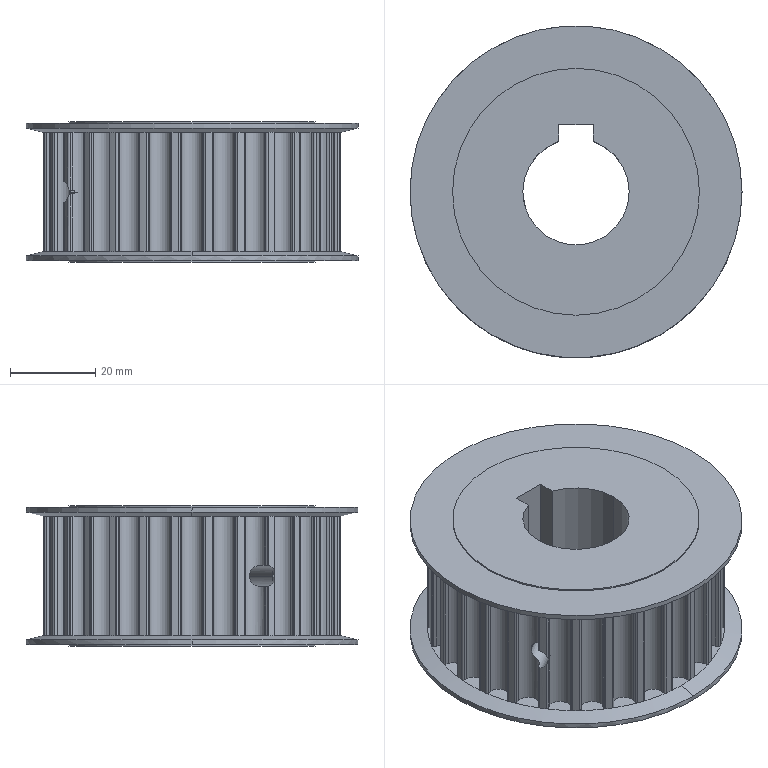Part | SolidWorks | features BaseBody 1 | 1 solid | 283 faces | box 78 x 78 x 33 mm | volume 99026 mm3 | cylinder 158 | plane 121 | cone 4 | commonest cylinder face diameters 0.81 x73 5.201 x41 69.93 x29 5 x4 58 x4 78 x4